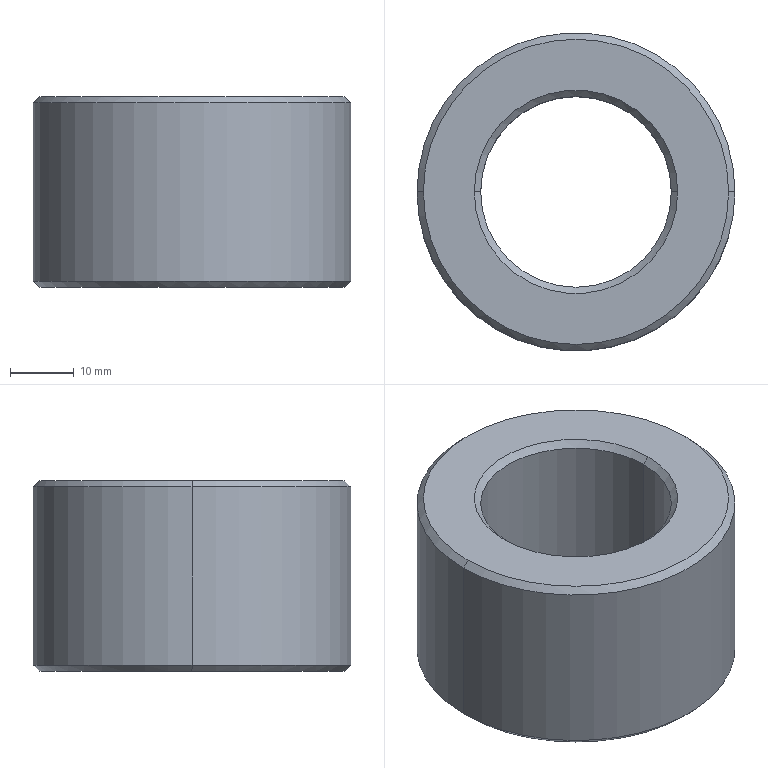Part | SolidWorks | features Chamfer 1, Extrusion 1 | 1 solid | 14 faces | box 50 x 50 x 30 mm | volume 37448 mm3 | cone 8 | cylinder 4 | plane 2 | commonest cylinder face diameters 30 x2 50 x2
STEP:
#1=CARTESIAN_POINT('',(24.,0.,30.));
#2=VERTEX_POINT('',#1);
#3=CARTESIAN_POINT('',(-24.,0.,30.));
#4=VERTEX_POINT('',#3);
#5=CARTESIAN_POINT('',(0.,0.,30.));
#6=DIRECTION('',(0.,0.,1.));
#7=DIRECTION('',(1.,0.,0.));
#8=AXIS2_PLACEMENT_3D('',#5,#6,#7);
#9=CIRCLE('',#8,24.);
#10=EDGE_CURVE('',#2,#4,#9,.T.);
#11=ORIENTED_EDGE('',*,*,#10,.F.);
#12=CARTESIAN_POINT('',(25.,0.,29.));
#13=VERTEX_POINT('',#12);
#14=CARTESIAN_POINT('',(24.,0.,30.));
#15=DIRECTION('',(0.7071,0.,-0.7071));
#16=VECTOR('',#15,1000.);
#17=LINE('',#14,#16);
#18=EDGE_CURVE('',#2,#13,#17,.T.);
#19=ORIENTED_EDGE('',*,*,#18,.T.);
#20=CARTESIAN_POINT('',(-25.,0.,29.));
#21=VERTEX_POINT('',#20);
#22=CARTESIAN_POINT('',(0.,0.,29.));
#23=DIRECTION('',(0.,0.,-1.));
#24=DIRECTION('',(1.,0.,0.));
#25=AXIS2_PLACEMENT_3D('',#22,#23,#24);
#26=CIRCLE('',#25,25.);
#27=EDGE_CURVE('',#21,#13,#26,.T.);
#28=ORIENTED_EDGE('',*,*,#27,.F.);
#29=CARTESIAN_POINT('',(-24.,0.,30.));
#30=DIRECTION('',(-0.7071,0.,-0.7071));
#31=VECTOR('',#30,1000.);
#32=LINE('',#29,#31);
#33=EDGE_CURVE('',#4,#21,#32,.T.);
#34=ORIENTED_EDGE('',*,*,#33,.F.);
#35=EDGE_LOOP('',(#11,#19,#28,#34));
#36=FACE_OUTER_BOUND('',#35,.T.);
#37=CARTESIAN_POINT('',(0.,0.,30.));
#38=DIRECTION('',(0.,0.,-1.));
#39=DIRECTION('',(-1.,0.,0.));
#40=AXIS2_PLACEMENT_3D('',#37,#38,#39);
#41=CONICAL_SURFACE('',#40,24.,0.7854);
#42=ADVANCED_FACE('',(#36),#41,.T.);
#43=CARTESIAN_POINT('',(-15.,0.,29.));
#44=VERTEX_POINT('',#43);
#45=CARTESIAN_POINT('',(15.,0.,29.));
#46=VERTEX_POINT('',#45);
#47=CARTESIAN_POINT('',(0.,0.,29.));
#48=DIRECTION('',(0.,0.,1.));
#49=DIRECTION('',(1.,0.,0.));
#50=AXIS2_PLACEMENT_3D('',#47,#48,#49);
#51=CIRCLE('',#50,15.);
#52=EDGE_CURVE('',#44,#46,#51,.T.);
#53=ORIENTED_EDGE('',*,*,#52,.F.);
#54=CARTESIAN_POINT('',(-16.,0.,30.));
#55=VERTEX_POINT('',#54);
#56=CARTESIAN_POINT('',(-15.,0.,29.));
#57=DIRECTION('',(-0.7071,0.,0.7071));
#58=VECTOR('',#57,1000.);
#59=LINE('',#56,#58);
#60=EDGE_CURVE('',#44,#55,#59,.T.);
#61=ORIENTED_EDGE('',*,*,#60,.T.);
#62=CARTESIAN_POINT('',(16.,0.,30.));
#63=VERTEX_POINT('',#62);
#64=CARTESIAN_POINT('',(0.,0.,30.));
#65=DIRECTION('',(0.,0.,-1.));
#66=DIRECTION('',(1.,0.,0.));
#67=AXIS2_PLACEMENT_3D('',#64,#65,#66);
#68=CIRCLE('',#67,16.);
#69=EDGE_CURVE('',#63,#55,#68,.T.);
#70=ORIENTED_EDGE('',*,*,#69,.F.);
#71=CARTESIAN_POINT('',(15.,0.,29.));
#72=DIRECTION('',(0.7071,0.,0.7071));
#73=VECTOR('',#72,1000.);
#74=LINE('',#71,#73);
#75=EDGE_CURVE('',#46,#63,#74,.T.);
#76=ORIENTED_EDGE('',*,*,#75,.F.);
#77=EDGE_LOOP('',(#53,#61,#70,#76));
#78=FACE_OUTER_BOUND('',#77,.T.);
#79=CARTESIAN_POINT('',(0.,0.,29.));
#80=DIRECTION('',(0.,0.,1.));
#81=DIRECTION('',(1.,0.,0.));
#82=AXIS2_PLACEMENT_3D('',#79,#80,#81);
#83=CONICAL_SURFACE('',#82,15.,0.7854);
#84=ADVANCED_FACE('',(#78),#83,.F.);
#85=CARTESIAN_POINT('',(-24.,0.,0.));
#86=VERTEX_POINT('',#85);
#87=CARTESIAN_POINT('',(24.,0.,0.));
#88=VERTEX_POINT('',#87);
#89=CARTESIAN_POINT('',(0.,0.,0.));
#90=DIRECTION('',(0.,0.,-1.));
#91=DIRECTION('',(1.,0.,0.));
#92=AXIS2_PLACEMENT_3D('',#89,#90,#91);
#93=CIRCLE('',#92,24.);
#94=EDGE_CURVE('',#86,#88,#93,.T.);
#95=ORIENTED_EDGE('',*,*,#94,.F.);
#96=CARTESIAN_POINT('',(-25.,0.,1.));
#97=VERTEX_POINT('',#96);
#98=CARTESIAN_POINT('',(-25.,0.,1.));
#99=DIRECTION('',(-0.7071,0.,0.7071));
#100=VECTOR('',#99,1000.);
#101=LINE('',#98,#100);
#102=EDGE_CURVE('',#86,#97,#101,.T.);
#103=ORIENTED_EDGE('',*,*,#102,.T.);
#104=CARTESIAN_POINT('',(25.,0.,1.));
#105=VERTEX_POINT('',#104);
#106=CARTESIAN_POINT('',(0.,0.,1.));
#107=DIRECTION('',(0.,0.,1.));
#108=DIRECTION('',(1.,0.,0.));
#109=AXIS2_PLACEMENT_3D('',#106,#107,#108);
#110=CIRCLE('',#109,25.);
#111=EDGE_CURVE('',#105,#97,#110,.T.);
#112=ORIENTED_EDGE('',*,*,#111,.F.);
#113=CARTESIAN_POINT('',(25.,0.,1.));
#114=DIRECTION('',(0.7071,0.,0.7071));
#115=VECTOR('',#114,1000.);
#116=LINE('',#113,#115);
#117=EDGE_CURVE('',#88,#105,#116,.T.);
#118=ORIENTED_EDGE('',*,*,#117,.F.);
#119=EDGE_LOOP('',(#95,#103,#112,#118));
#120=FACE_OUTER_BOUND('',#119,.T.);
#121=CARTESIAN_POINT('',(0.,0.,1.));
#122=DIRECTION('',(0.,0.,1.));
#123=DIRECTION('',(1.,0.,0.));
#124=AXIS2_PLACEMENT_3D('',#121,#122,#123);
#125=CONICAL_SURFACE('',#124,25.,0.7854);
#126=ADVANCED_FACE('',(#120),#125,.T.);
#127=CARTESIAN_POINT('',(15.,0.,1.));
#128=VERTEX_POINT('',#127);
#129=CARTESIAN_POINT('',(-15.,0.,1.));
#130=VERTEX_POINT('',#129);
#131=CARTESIAN_POINT('',(0.,0.,1.));
#132=DIRECTION('',(0.,0.,-1.));
#133=DIRECTION('',(1.,0.,0.));
#134=AXIS2_PLACEMENT_3D('',#131,#132,#133);
#135=CIRCLE('',#134,15.);
#136=EDGE_CURVE('',#128,#130,#135,.T.);
#137=ORIENTED_EDGE('',*,*,#136,.F.);
#138=CARTESIAN_POINT('',(16.,0.,0.));
#139=VERTEX_POINT('',#138);
#140=CARTESIAN_POINT('',(16.,0.,0.));
#141=DIRECTION('',(0.7071,0.,-0.7071));
#142=VECTOR('',#141,1000.);
#143=LINE('',#140,#142);
#144=EDGE_CURVE('',#128,#139,#143,.T.);
#145=ORIENTED_EDGE('',*,*,#144,.T.);
#146=CARTESIAN_POINT('',(-16.,0.,0.));
#147=VERTEX_POINT('',#146);
#148=CARTESIAN_POINT('',(0.,0.,0.));
#149=DIRECTION('',(0.,0.,1.));
#150=DIRECTION('',(1.,0.,0.));
#151=AXIS2_PLACEMENT_3D('',#148,#149,#150);
#152=CIRCLE('',#151,16.);
#153=EDGE_CURVE('',#147,#139,#152,.T.);
#154=ORIENTED_EDGE('',*,*,#153,.F.);
#155=CARTESIAN_POINT('',(-16.,0.,0.));
#156=DIRECTION('',(-0.7071,0.,-0.7071));
#157=VECTOR('',#156,1000.);
#158=LINE('',#155,#157);
#159=EDGE_CURVE('',#130,#147,#158,.T.);
#160=ORIENTED_EDGE('',*,*,#159,.F.);
#161=EDGE_LOOP('',(#137,#145,#154,#160));
#162=FACE_OUTER_BOUND('',#161,.T.);
#163=CARTESIAN_POINT('',(0.,0.,0.));
#164=DIRECTION('',(0.,0.,-1.));
#165=DIRECTION('',(-1.,0.,0.));
#166=AXIS2_PLACEMENT_3D('',#163,#164,#165);
#167=CONICAL_SURFACE('',#166,16.,0.7854);
#168=ADVANCED_FACE('',(#162),#167,.F.);
#169=ORIENTED_EDGE('',*,*,#52,.T.);
#170=CARTESIAN_POINT('',(15.,0.,30.));
#171=DIRECTION('',(0.,0.,-1.));
#172=VECTOR('',#171,1000.);
#173=LINE('',#170,#172);
#174=EDGE_CURVE('',#46,#128,#173,.T.);
#175=ORIENTED_EDGE('',*,*,#174,.T.);
#176=ORIENTED_EDGE('',*,*,#136,.T.);
#177=CARTESIAN_POINT('',(-15.,0.,30.));
#178=DIRECTION('',(0.,0.,-1.));
#179=VECTOR('',#178,1000.);
#180=LINE('',#177,#179);
#181=EDGE_CURVE('',#44,#130,#180,.T.);
#182=ORIENTED_EDGE('',*,*,#181,.F.);
#183=EDGE_LOOP('',(#169,#175,#176,#182));
#184=FACE_OUTER_BOUND('',#183,.T.);
#185=CARTESIAN_POINT('',(0.,0.,30.));
#186=DIRECTION('',(0.,0.,-1.));
#187=DIRECTION('',(-1.,0.,0.));
#188=AXIS2_PLACEMENT_3D('',#185,#186,#187);
#189=CYLINDRICAL_SURFACE('',#188,15.);
#190=ADVANCED_FACE('',(#184),#189,.F.);
#191=ORIENTED_EDGE('',*,*,#27,.T.);
#192=CARTESIAN_POINT('',(25.,0.,30.));
#193=DIRECTION('',(0.,0.,-1.));
#194=VECTOR('',#193,1000.);
#195=LINE('',#192,#194);
#196=EDGE_CURVE('',#13,#105,#195,.T.);
#197=ORIENTED_EDGE('',*,*,#196,.T.);
#198=ORIENTED_EDGE('',*,*,#111,.T.);
#199=CARTESIAN_POINT('',(-25.,0.,30.));
#200=DIRECTION('',(0.,0.,-1.));
#201=VECTOR('',#200,1000.);
#202=LINE('',#199,#201);
#203=EDGE_CURVE('',#21,#97,#202,.T.);
#204=ORIENTED_EDGE('',*,*,#203,.F.);
#205=EDGE_LOOP('',(#191,#197,#198,#204));
#206=FACE_OUTER_BOUND('',#205,.T.);
#207=CARTESIAN_POINT('',(0.,0.,30.));
#208=DIRECTION('',(0.,0.,-1.));
#209=DIRECTION('',(-1.,0.,0.));
#210=AXIS2_PLACEMENT_3D('',#207,#208,#209);
#211=CYLINDRICAL_SURFACE('',#210,25.);
#212=ADVANCED_FACE('',(#206),#211,.T.);
#213=ORIENTED_EDGE('',*,*,#69,.T.);
#214=CARTESIAN_POINT('',(0.,0.,30.));
#215=DIRECTION('',(0.,0.,-1.));
#216=DIRECTION('',(1.,0.,0.));
#217=AXIS2_PLACEMENT_3D('',#214,#215,#216);
#218=CIRCLE('',#217,16.);
#219=EDGE_CURVE('',#55,#63,#218,.T.);
#220=ORIENTED_EDGE('',*,*,#219,.T.);
#221=EDGE_LOOP('',(#213,#220));
#222=FACE_BOUND('',#221,.T.);
#223=CARTESIAN_POINT('',(0.,0.,30.));
#224=DIRECTION('',(0.,0.,1.));
#225=DIRECTION('',(1.,0.,0.));
#226=AXIS2_PLACEMENT_3D('',#223,#224,#225);
#227=CIRCLE('',#226,24.);
#228=EDGE_CURVE('',#4,#2,#227,.T.);
#229=ORIENTED_EDGE('',*,*,#228,.T.);
#230=ORIENTED_EDGE('',*,*,#10,.T.);
#231=EDGE_LOOP('',(#229,#230));
#232=FACE_OUTER_BOUND('',#231,.T.);
#233=CARTESIAN_POINT('',(0.,0.,30.));
#234=DIRECTION('',(0.,0.,1.));
#235=DIRECTION('',(1.,0.,0.));
#236=AXIS2_PLACEMENT_3D('',#233,#234,#235);
#237=PLANE('',#236);
#238=ADVANCED_FACE('',(#222,#232),#237,.T.);
#239=ORIENTED_EDGE('',*,*,#153,.T.);
#240=CARTESIAN_POINT('',(0.,0.,0.));
#241=DIRECTION('',(0.,0.,1.));
#242=DIRECTION('',(1.,0.,0.));
#243=AXIS2_PLACEMENT_3D('',#240,#241,#242);
#244=CIRCLE('',#243,16.);
#245=EDGE_CURVE('',#139,#147,#244,.T.);
#246=ORIENTED_EDGE('',*,*,#245,.T.);
#247=EDGE_LOOP('',(#239,#246));
#248=FACE_BOUND('',#247,.T.);
#249=CARTESIAN_POINT('',(0.,0.,0.));
#250=DIRECTION('',(0.,0.,-1.));
#251=DIRECTION('',(1.,0.,0.));
#252=AXIS2_PLACEMENT_3D('',#249,#250,#251);
#253=CIRCLE('',#252,24.);
#254=EDGE_CURVE('',#88,#86,#253,.T.);
#255=ORIENTED_EDGE('',*,*,#254,.T.);
#256=ORIENTED_EDGE('',*,*,#94,.T.);
#257=EDGE_LOOP('',(#255,#256));
#258=FACE_OUTER_BOUND('',#257,.T.);
#259=CARTESIAN_POINT('',(0.,0.,0.));
#260=DIRECTION('',(0.,0.,1.));
#261=DIRECTION('',(1.,0.,0.));
#262=AXIS2_PLACEMENT_3D('',#259,#260,#261);
#263=PLANE('',#262);
#264=ADVANCED_FACE('',(#248,#258),#263,.F.);
#265=ORIENTED_EDGE('',*,*,#196,.F.);
#266=CARTESIAN_POINT('',(0.,0.,29.));
#267=DIRECTION('',(0.,0.,-1.));
#268=DIRECTION('',(1.,0.,0.));
#269=AXIS2_PLACEMENT_3D('',#266,#267,#268);
#270=CIRCLE('',#269,25.);
#271=EDGE_CURVE('',#13,#21,#270,.T.);
#272=ORIENTED_EDGE('',*,*,#271,.T.);
#273=ORIENTED_EDGE('',*,*,#203,.T.);
#274=CARTESIAN_POINT('',(0.,0.,1.));
#275=DIRECTION('',(0.,0.,1.));
#276=DIRECTION('',(1.,0.,0.));
#277=AXIS2_PLACEMENT_3D('',#274,#275,#276);
#278=CIRCLE('',#277,25.);
#279=EDGE_CURVE('',#97,#105,#278,.T.);
#280=ORIENTED_EDGE('',*,*,#279,.T.);
#281=EDGE_LOOP('',(#265,#272,#273,#280));
#282=FACE_OUTER_BOUND('',#281,.T.);
#283=CARTESIAN_POINT('',(0.,0.,30.));
#284=DIRECTION('',(0.,0.,-1.));
#285=DIRECTION('',(-1.,0.,0.));
#286=AXIS2_PLACEMENT_3D('',#283,#284,#285);
#287=CYLINDRICAL_SURFACE('',#286,25.);
#288=ADVANCED_FACE('',(#282),#287,.T.);
#289=ORIENTED_EDGE('',*,*,#174,.F.);
#290=CARTESIAN_POINT('',(0.,0.,29.));
#291=DIRECTION('',(0.,0.,1.));
#292=DIRECTION('',(1.,0.,0.));
#293=AXIS2_PLACEMENT_3D('',#290,#291,#292);
#294=CIRCLE('',#293,15.);
#295=EDGE_CURVE('',#46,#44,#294,.T.);
#296=ORIENTED_EDGE('',*,*,#295,.T.);
#297=ORIENTED_EDGE('',*,*,#181,.T.);
#298=CARTESIAN_POINT('',(0.,0.,1.));
#299=DIRECTION('',(0.,0.,-1.));
#300=DIRECTION('',(1.,0.,0.));
#301=AXIS2_PLACEMENT_3D('',#298,#299,#300);
#302=CIRCLE('',#301,15.);
#303=EDGE_CURVE('',#130,#128,#302,.T.);
#304=ORIENTED_EDGE('',*,*,#303,.T.);
#305=EDGE_LOOP('',(#289,#296,#297,#304));
#306=FACE_OUTER_BOUND('',#305,.T.);
#307=CARTESIAN_POINT('',(0.,0.,30.));
#308=DIRECTION('',(0.,0.,-1.));
#309=DIRECTION('',(-1.,0.,0.));
#310=AXIS2_PLACEMENT_3D('',#307,#308,#309);
#311=CYLINDRICAL_SURFACE('',#310,15.);
#312=ADVANCED_FACE('',(#306),#311,.F.);
#313=ORIENTED_EDGE('',*,*,#144,.F.);
#314=ORIENTED_EDGE('',*,*,#303,.F.);
#315=ORIENTED_EDGE('',*,*,#159,.T.);
#316=ORIENTED_EDGE('',*,*,#245,.F.);
#317=EDGE_LOOP('',(#313,#314,#315,#316));
#318=FACE_OUTER_BOUND('',#317,.T.);
#319=CARTESIAN_POINT('',(0.,0.,0.));
#320=DIRECTION('',(0.,0.,-1.));
#321=DIRECTION('',(-1.,0.,0.));
#322=AXIS2_PLACEMENT_3D('',#319,#320,#321);
#323=CONICAL_SURFACE('',#322,16.,0.7854);
#324=ADVANCED_FACE('',(#318),#323,.F.);
#325=ORIENTED_EDGE('',*,*,#102,.F.);
#326=ORIENTED_EDGE('',*,*,#254,.F.);
#327=ORIENTED_EDGE('',*,*,#117,.T.);
#328=ORIENTED_EDGE('',*,*,#279,.F.);
#329=EDGE_LOOP('',(#325,#326,#327,#328));
#330=FACE_OUTER_BOUND('',#329,.T.);
#331=CARTESIAN_POINT('',(0.,0.,1.));
#332=DIRECTION('',(0.,0.,1.));
#333=DIRECTION('',(1.,0.,0.));
#334=AXIS2_PLACEMENT_3D('',#331,#332,#333);
#335=CONICAL_SURFACE('',#334,25.,0.7854);
#336=ADVANCED_FACE('',(#330),#335,.T.);
#337=ORIENTED_EDGE('',*,*,#60,.F.);
#338=ORIENTED_EDGE('',*,*,#295,.F.);
#339=ORIENTED_EDGE('',*,*,#75,.T.);
#340=ORIENTED_EDGE('',*,*,#219,.F.);
#341=EDGE_LOOP('',(#337,#338,#339,#340));
#342=FACE_OUTER_BOUND('',#341,.T.);
#343=CARTESIAN_POINT('',(0.,0.,29.));
#344=DIRECTION('',(0.,0.,1.));
#345=DIRECTION('',(1.,0.,0.));
#346=AXIS2_PLACEMENT_3D('',#343,#344,#345);
#347=CONICAL_SURFACE('',#346,15.,0.7854);
#348=ADVANCED_FACE('',(#342),#347,.F.);
#349=ORIENTED_EDGE('',*,*,#18,.F.);
#350=ORIENTED_EDGE('',*,*,#228,.F.);
#351=ORIENTED_EDGE('',*,*,#33,.T.);
#352=ORIENTED_EDGE('',*,*,#271,.F.);
#353=EDGE_LOOP('',(#349,#350,#351,#352));
#354=FACE_OUTER_BOUND('',#353,.T.);
#355=CARTESIAN_POINT('',(0.,0.,30.));
#356=DIRECTION('',(0.,0.,-1.));
#357=DIRECTION('',(-1.,0.,0.));
#358=AXIS2_PLACEMENT_3D('',#355,#356,#357);
#359=CONICAL_SURFACE('',#358,24.,0.7854);
#360=ADVANCED_FACE('',(#354),#359,.T.);
#361=CLOSED_SHELL('',(#42,#84,#126,#168,#190,#212,#238,#264,#288,#312,#324,#336,#348,#360));
#362=MANIFOLD_SOLID_BREP('',#361);
#363=CARTESIAN_POINT('',(0.,0.,0.));
#364=DIRECTION('',(0.,0.,1.));
#365=DIRECTION('',(1.,0.,0.));
#366=AXIS2_PLACEMENT_3D('',#363,#364,#365);
#367=(LENGTH_UNIT()NAMED_UNIT(*)SI_UNIT(.MILLI.,.METRE.));
#368=UNCERTAINTY_MEASURE_WITH_UNIT(LENGTH_MEASURE(0.00001),#367,'','');
#369=(NAMED_UNIT(*)PLANE_ANGLE_UNIT()SI_UNIT($,.RADIAN.));
#370=(NAMED_UNIT(*)SI_UNIT($,.STERADIAN.)SOLID_ANGLE_UNIT());
#371=(GEOMETRIC_REPRESENTATION_CONTEXT(3)GLOBAL_UNCERTAINTY_ASSIGNED_CONTEXT((#368))GLOBAL_UNIT_ASSIGNED_CONTEXT((#367,#369,#370))REPRESENTATION_CONTEXT('',''));
#372=ADVANCED_BREP_SHAPE_REPRESENTATION('',(#362,#366),#371);